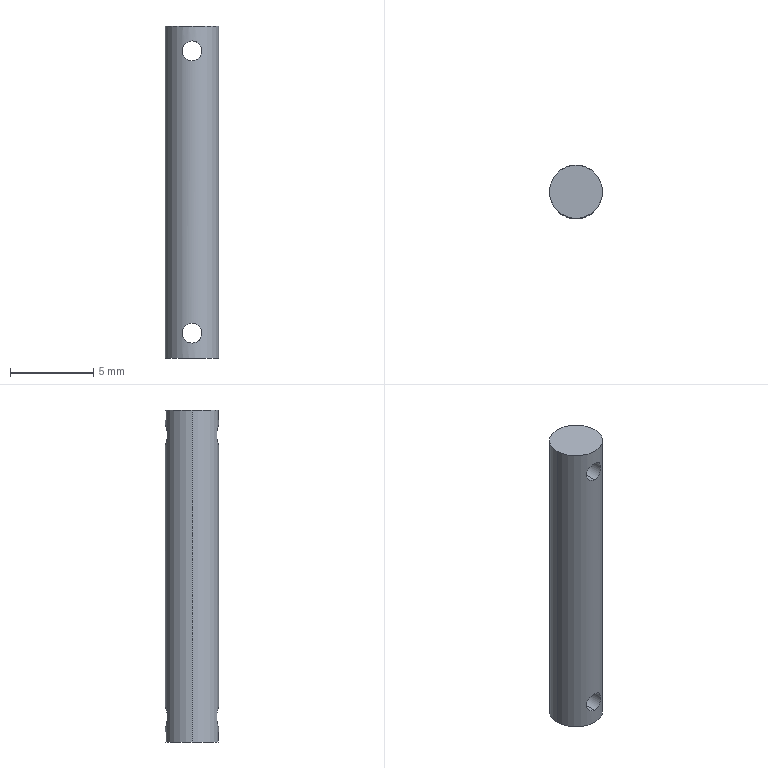Part | SolidWorks | features BaseBody 1 | 1 solid | 8 faces | box 3.2 x 3.2 x 20 mm | volume 153.742 mm3 | cylinder 6 | plane 2 | commonest cylinder face diameters 1.2 x4 3.2 x2
STEP:
#1=CARTESIAN_POINT('',(0.,-1.6,0.9));
#2=VERTEX_POINT('',#1);
#3=CARTESIAN_POINT('',(0.,1.6,0.9));
#4=VERTEX_POINT('',#3);
#5=CARTESIAN_POINT('',(0.,-1.6,0.9));
#6=DIRECTION('',(0.,1.,0.));
#7=VECTOR('',#6,1000.);
#8=LINE('',#5,#7);
#9=EDGE_CURVE('',#2,#4,#8,.T.);
#10=ORIENTED_EDGE('',*,*,#9,.F.);
#11=CARTESIAN_POINT('',(0.,-1.6,2.1));
#12=VERTEX_POINT('',#11);
#13=CARTESIAN_POINT('',(0.,-1.6,2.1));
#14=CARTESIAN_POINT('',(0.0792,-1.6,2.1));
#15=CARTESIAN_POINT('',(0.1577,-1.594,2.084));
#16=CARTESIAN_POINT('',(0.3049,-1.572,2.022));
#17=CARTESIAN_POINT('',(0.3691,-1.558,1.979));
#18=CARTESIAN_POINT('',(0.4799,-1.527,1.869));
#19=CARTESIAN_POINT('',(0.5219,-1.513,1.806));
#20=CARTESIAN_POINT('',(0.5845,-1.49,1.655));
#21=CARTESIAN_POINT('',(0.5999,-1.483,1.578));
#22=CARTESIAN_POINT('',(0.6001,-1.483,1.422));
#23=CARTESIAN_POINT('',(0.584,-1.49,1.344));
#24=CARTESIAN_POINT('',(0.5225,-1.513,1.196));
#25=CARTESIAN_POINT('',(0.48,-1.527,1.131));
#26=CARTESIAN_POINT('',(0.3682,-1.558,1.02));
#27=CARTESIAN_POINT('',(0.3045,-1.573,0.9769));
#28=CARTESIAN_POINT('',(0.1569,-1.594,0.9154));
#29=CARTESIAN_POINT('',(0.07976,-1.6,0.9));
#30=CARTESIAN_POINT('',(0.,-1.6,0.9));
#31=B_SPLINE_CURVE_WITH_KNOTS('',3,(#13,#14,#15,#16,#17,#18,#19,#20,#21,#22,#23,#24,#25,#26,#27,#28,#29,#30),.UNSPECIFIED.,.F.,.F.,(4,2,2,2,2,2,2,2,4),(0.,0.125,0.25,0.375,0.5,0.625,0.75,0.875,1.),.UNSPECIFIED.);
#32=EDGE_CURVE('',#12,#2,#31,.T.);
#33=ORIENTED_EDGE('',*,*,#32,.F.);
#34=CARTESIAN_POINT('',(0.,1.6,2.1));
#35=VERTEX_POINT('',#34);
#36=CARTESIAN_POINT('',(0.,-1.6,2.1));
#37=DIRECTION('',(0.,1.,0.));
#38=VECTOR('',#37,1000.);
#39=LINE('',#36,#38);
#40=EDGE_CURVE('',#12,#35,#39,.T.);
#41=ORIENTED_EDGE('',*,*,#40,.T.);
#42=CARTESIAN_POINT('',(0.,1.6,0.9));
#43=CARTESIAN_POINT('',(0.07978,1.6,0.9));
#44=CARTESIAN_POINT('',(0.1578,1.594,0.9157));
#45=CARTESIAN_POINT('',(0.304,1.573,0.9767));
#46=CARTESIAN_POINT('',(0.3682,1.558,1.02));
#47=CARTESIAN_POINT('',(0.4809,1.527,1.132));
#48=CARTESIAN_POINT('',(0.5232,1.512,1.195));
#49=CARTESIAN_POINT('',(0.5848,1.49,1.344));
#50=CARTESIAN_POINT('',(0.6,1.483,1.422));
#51=CARTESIAN_POINT('',(0.6,1.483,1.578));
#52=CARTESIAN_POINT('',(0.5839,1.49,1.657));
#53=CARTESIAN_POINT('',(0.5225,1.513,1.804));
#54=CARTESIAN_POINT('',(0.4795,1.528,1.869));
#55=CARTESIAN_POINT('',(0.3687,1.558,1.98));
#56=CARTESIAN_POINT('',(0.3053,1.572,2.022));
#57=CARTESIAN_POINT('',(0.1565,1.594,2.084));
#58=CARTESIAN_POINT('',(0.07933,1.6,2.1));
#59=CARTESIAN_POINT('',(0.,1.6,2.1));
#60=B_SPLINE_CURVE_WITH_KNOTS('',3,(#42,#43,#44,#45,#46,#47,#48,#49,#50,#51,#52,#53,#54,#55,#56,#57,#58,#59),.UNSPECIFIED.,.F.,.F.,(4,2,2,2,2,2,2,2,4),(0.,0.125,0.25,0.375,0.5,0.625,0.75,0.875,1.),.UNSPECIFIED.);
#61=EDGE_CURVE('',#4,#35,#60,.T.);
#62=ORIENTED_EDGE('',*,*,#61,.F.);
#63=EDGE_LOOP('',(#10,#33,#41,#62));
#64=FACE_OUTER_BOUND('',#63,.T.);
#65=CARTESIAN_POINT('',(0.,-1.6,1.5));
#66=DIRECTION('',(0.,1.,0.));
#67=DIRECTION('',(0.,0.,1.));
#68=AXIS2_PLACEMENT_3D('',#65,#66,#67);
#69=CYLINDRICAL_SURFACE('',#68,0.6);
#70=ADVANCED_FACE('',(#64),#69,.F.);
#71=CARTESIAN_POINT('',(0.,-1.6,17.9));
#72=VERTEX_POINT('',#71);
#73=CARTESIAN_POINT('',(0.,1.6,17.9));
#74=VERTEX_POINT('',#73);
#75=CARTESIAN_POINT('',(0.,-1.6,17.9));
#76=DIRECTION('',(0.,1.,0.));
#77=VECTOR('',#76,1000.);
#78=LINE('',#75,#77);
#79=EDGE_CURVE('',#72,#74,#78,.T.);
#80=ORIENTED_EDGE('',*,*,#79,.F.);
#81=CARTESIAN_POINT('',(0.,-1.6,19.1));
#82=VERTEX_POINT('',#81);
#83=CARTESIAN_POINT('',(0.,-1.6,19.1));
#84=CARTESIAN_POINT('',(0.0792,-1.6,19.1));
#85=CARTESIAN_POINT('',(0.1577,-1.594,19.084));
#86=CARTESIAN_POINT('',(0.3049,-1.572,19.022));
#87=CARTESIAN_POINT('',(0.3691,-1.558,18.979));
#88=CARTESIAN_POINT('',(0.4799,-1.527,18.869));
#89=CARTESIAN_POINT('',(0.5219,-1.513,18.806));
#90=CARTESIAN_POINT('',(0.5845,-1.49,18.655));
#91=CARTESIAN_POINT('',(0.5999,-1.483,18.578));
#92=CARTESIAN_POINT('',(0.6001,-1.483,18.422));
#93=CARTESIAN_POINT('',(0.584,-1.49,18.344));
#94=CARTESIAN_POINT('',(0.5225,-1.513,18.196));
#95=CARTESIAN_POINT('',(0.48,-1.527,18.131));
#96=CARTESIAN_POINT('',(0.3682,-1.558,18.02));
#97=CARTESIAN_POINT('',(0.3045,-1.573,17.977));
#98=CARTESIAN_POINT('',(0.1569,-1.594,17.915));
#99=CARTESIAN_POINT('',(0.07976,-1.6,17.9));
#100=CARTESIAN_POINT('',(0.,-1.6,17.9));
#101=B_SPLINE_CURVE_WITH_KNOTS('',3,(#83,#84,#85,#86,#87,#88,#89,#90,#91,#92,#93,#94,#95,#96,#97,#98,#99,#100),.UNSPECIFIED.,.F.,.F.,(4,2,2,2,2,2,2,2,4),(0.,0.125,0.25,0.375,0.5,0.625,0.75,0.875,1.),.UNSPECIFIED.);
#102=EDGE_CURVE('',#82,#72,#101,.T.);
#103=ORIENTED_EDGE('',*,*,#102,.F.);
#104=CARTESIAN_POINT('',(0.,1.6,19.1));
#105=VERTEX_POINT('',#104);
#106=CARTESIAN_POINT('',(0.,-1.6,19.1));
#107=DIRECTION('',(0.,1.,0.));
#108=VECTOR('',#107,1000.);
#109=LINE('',#106,#108);
#110=EDGE_CURVE('',#82,#105,#109,.T.);
#111=ORIENTED_EDGE('',*,*,#110,.T.);
#112=CARTESIAN_POINT('',(0.,1.6,17.9));
#113=CARTESIAN_POINT('',(0.07978,1.6,17.9));
#114=CARTESIAN_POINT('',(0.1578,1.594,17.916));
#115=CARTESIAN_POINT('',(0.304,1.573,17.977));
#116=CARTESIAN_POINT('',(0.3682,1.558,18.02));
#117=CARTESIAN_POINT('',(0.4809,1.527,18.132));
#118=CARTESIAN_POINT('',(0.5232,1.512,18.195));
#119=CARTESIAN_POINT('',(0.5848,1.49,18.344));
#120=CARTESIAN_POINT('',(0.6,1.483,18.422));
#121=CARTESIAN_POINT('',(0.6,1.483,18.578));
#122=CARTESIAN_POINT('',(0.5839,1.49,18.657));
#123=CARTESIAN_POINT('',(0.5225,1.513,18.804));
#124=CARTESIAN_POINT('',(0.4795,1.528,18.869));
#125=CARTESIAN_POINT('',(0.3687,1.558,18.98));
#126=CARTESIAN_POINT('',(0.3053,1.572,19.022));
#127=CARTESIAN_POINT('',(0.1565,1.594,19.084));
#128=CARTESIAN_POINT('',(0.07933,1.6,19.1));
#129=CARTESIAN_POINT('',(0.,1.6,19.1));
#130=B_SPLINE_CURVE_WITH_KNOTS('',3,(#112,#113,#114,#115,#116,#117,#118,#119,#120,#121,#122,#123,#124,#125,#126,#127,#128,#129),.UNSPECIFIED.,.F.,.F.,(4,2,2,2,2,2,2,2,4),(0.,0.125,0.25,0.375,0.5,0.625,0.75,0.875,1.),.UNSPECIFIED.);
#131=EDGE_CURVE('',#74,#105,#130,.T.);
#132=ORIENTED_EDGE('',*,*,#131,.F.);
#133=EDGE_LOOP('',(#80,#103,#111,#132));
#134=FACE_OUTER_BOUND('',#133,.T.);
#135=CARTESIAN_POINT('',(0.,-1.6,18.5));
#136=DIRECTION('',(0.,1.,0.));
#137=DIRECTION('',(0.,0.,1.));
#138=AXIS2_PLACEMENT_3D('',#135,#136,#137);
#139=CYLINDRICAL_SURFACE('',#138,0.6);
#140=ADVANCED_FACE('',(#134),#139,.F.);
#141=CARTESIAN_POINT('',(-1.6,0.,0.));
#142=VERTEX_POINT('',#141);
#143=CARTESIAN_POINT('',(1.6,0.,0.));
#144=VERTEX_POINT('',#143);
#145=CARTESIAN_POINT('',(0.,0.,0.));
#146=DIRECTION('',(0.,0.,1.));
#147=DIRECTION('',(1.,0.,0.));
#148=AXIS2_PLACEMENT_3D('',#145,#146,#147);
#149=CIRCLE('',#148,1.6);
#150=EDGE_CURVE('',#142,#144,#149,.T.);
#151=ORIENTED_EDGE('',*,*,#150,.F.);
#152=CARTESIAN_POINT('',(0.,0.,0.));
#153=DIRECTION('',(0.,0.,1.));
#154=DIRECTION('',(1.,0.,0.));
#155=AXIS2_PLACEMENT_3D('',#152,#153,#154);
#156=CIRCLE('',#155,1.6);
#157=EDGE_CURVE('',#144,#142,#156,.T.);
#158=ORIENTED_EDGE('',*,*,#157,.F.);
#159=EDGE_LOOP('',(#151,#158));
#160=FACE_OUTER_BOUND('',#159,.T.);
#161=CARTESIAN_POINT('',(0.,0.,0.));
#162=DIRECTION('',(0.,0.,1.));
#163=DIRECTION('',(1.,0.,0.));
#164=AXIS2_PLACEMENT_3D('',#161,#162,#163);
#165=PLANE('',#164);
#166=ADVANCED_FACE('',(#160),#165,.F.);
#167=CARTESIAN_POINT('',(-1.6,0.,20.));
#168=VERTEX_POINT('',#167);
#169=CARTESIAN_POINT('',(1.6,0.,20.));
#170=VERTEX_POINT('',#169);
#171=CARTESIAN_POINT('',(0.,0.,20.));
#172=DIRECTION('',(0.,0.,1.));
#173=DIRECTION('',(1.,0.,0.));
#174=AXIS2_PLACEMENT_3D('',#171,#172,#173);
#175=CIRCLE('',#174,1.6);
#176=EDGE_CURVE('',#168,#170,#175,.T.);
#177=ORIENTED_EDGE('',*,*,#176,.T.);
#178=CARTESIAN_POINT('',(0.,0.,20.));
#179=DIRECTION('',(0.,0.,1.));
#180=DIRECTION('',(1.,0.,0.));
#181=AXIS2_PLACEMENT_3D('',#178,#179,#180);
#182=CIRCLE('',#181,1.6);
#183=EDGE_CURVE('',#170,#168,#182,.T.);
#184=ORIENTED_EDGE('',*,*,#183,.T.);
#185=EDGE_LOOP('',(#177,#184));
#186=FACE_OUTER_BOUND('',#185,.T.);
#187=CARTESIAN_POINT('',(0.,0.,20.));
#188=DIRECTION('',(0.,0.,1.));
#189=DIRECTION('',(1.,0.,0.));
#190=AXIS2_PLACEMENT_3D('',#187,#188,#189);
#191=PLANE('',#190);
#192=ADVANCED_FACE('',(#186),#191,.T.);
#193=ORIENTED_EDGE('',*,*,#102,.T.);
#194=CARTESIAN_POINT('',(0.,-1.6,17.9));
#195=CARTESIAN_POINT('',(-0.07978,-1.6,17.9));
#196=CARTESIAN_POINT('',(-0.1578,-1.594,17.916));
#197=CARTESIAN_POINT('',(-0.304,-1.573,17.977));
#198=CARTESIAN_POINT('',(-0.3682,-1.558,18.02));
#199=CARTESIAN_POINT('',(-0.4809,-1.527,18.132));
#200=CARTESIAN_POINT('',(-0.5232,-1.512,18.195));
#201=CARTESIAN_POINT('',(-0.5848,-1.49,18.344));
#202=CARTESIAN_POINT('',(-0.6,-1.483,18.422));
#203=CARTESIAN_POINT('',(-0.6,-1.483,18.578));
#204=CARTESIAN_POINT('',(-0.5839,-1.49,18.657));
#205=CARTESIAN_POINT('',(-0.5225,-1.513,18.804));
#206=CARTESIAN_POINT('',(-0.4795,-1.528,18.869));
#207=CARTESIAN_POINT('',(-0.3687,-1.558,18.98));
#208=CARTESIAN_POINT('',(-0.3053,-1.572,19.022));
#209=CARTESIAN_POINT('',(-0.1565,-1.594,19.084));
#210=CARTESIAN_POINT('',(-0.07933,-1.6,19.1));
#211=CARTESIAN_POINT('',(0.,-1.6,19.1));
#212=B_SPLINE_CURVE_WITH_KNOTS('',3,(#194,#195,#196,#197,#198,#199,#200,#201,#202,#203,#204,#205,#206,#207,#208,#209,#210,#211),.UNSPECIFIED.,.F.,.F.,(4,2,2,2,2,2,2,2,4),(0.,0.125,0.25,0.375,0.5,0.625,0.75,0.875,1.),.UNSPECIFIED.);
#213=EDGE_CURVE('',#72,#82,#212,.T.);
#214=ORIENTED_EDGE('',*,*,#213,.T.);
#215=EDGE_LOOP('',(#193,#214));
#216=FACE_BOUND('',#215,.T.);
#217=ORIENTED_EDGE('',*,*,#32,.T.);
#218=CARTESIAN_POINT('',(0.,-1.6,0.9));
#219=CARTESIAN_POINT('',(-0.07978,-1.6,0.9));
#220=CARTESIAN_POINT('',(-0.1578,-1.594,0.9157));
#221=CARTESIAN_POINT('',(-0.304,-1.573,0.9767));
#222=CARTESIAN_POINT('',(-0.3682,-1.558,1.02));
#223=CARTESIAN_POINT('',(-0.4809,-1.527,1.132));
#224=CARTESIAN_POINT('',(-0.5232,-1.512,1.195));
#225=CARTESIAN_POINT('',(-0.5848,-1.49,1.344));
#226=CARTESIAN_POINT('',(-0.6,-1.483,1.422));
#227=CARTESIAN_POINT('',(-0.6,-1.483,1.578));
#228=CARTESIAN_POINT('',(-0.5839,-1.49,1.657));
#229=CARTESIAN_POINT('',(-0.5225,-1.513,1.804));
#230=CARTESIAN_POINT('',(-0.4795,-1.528,1.869));
#231=CARTESIAN_POINT('',(-0.3687,-1.558,1.98));
#232=CARTESIAN_POINT('',(-0.3053,-1.572,2.022));
#233=CARTESIAN_POINT('',(-0.1565,-1.594,2.084));
#234=CARTESIAN_POINT('',(-0.07933,-1.6,2.1));
#235=CARTESIAN_POINT('',(0.,-1.6,2.1));
#236=B_SPLINE_CURVE_WITH_KNOTS('',3,(#218,#219,#220,#221,#222,#223,#224,#225,#226,#227,#228,#229,#230,#231,#232,#233,#234,#235),.UNSPECIFIED.,.F.,.F.,(4,2,2,2,2,2,2,2,4),(0.,0.125,0.25,0.375,0.5,0.625,0.75,0.875,1.),.UNSPECIFIED.);
#237=EDGE_CURVE('',#2,#12,#236,.T.);
#238=ORIENTED_EDGE('',*,*,#237,.T.);
#239=EDGE_LOOP('',(#217,#238));
#240=FACE_BOUND('',#239,.T.);
#241=CARTESIAN_POINT('',(1.6,0.,20.));
#242=DIRECTION('',(0.,0.,-1.));
#243=VECTOR('',#242,1000.);
#244=LINE('',#241,#243);
#245=EDGE_CURVE('',#170,#144,#244,.T.);
#246=ORIENTED_EDGE('',*,*,#245,.F.);
#247=ORIENTED_EDGE('',*,*,#176,.F.);
#248=CARTESIAN_POINT('',(-1.6,0.,20.));
#249=DIRECTION('',(0.,0.,-1.));
#250=VECTOR('',#249,1000.);
#251=LINE('',#248,#250);
#252=EDGE_CURVE('',#168,#142,#251,.T.);
#253=ORIENTED_EDGE('',*,*,#252,.T.);
#254=ORIENTED_EDGE('',*,*,#150,.T.);
#255=EDGE_LOOP('',(#246,#247,#253,#254));
#256=FACE_OUTER_BOUND('',#255,.T.);
#257=CARTESIAN_POINT('',(0.,0.,20.));
#258=DIRECTION('',(0.,0.,-1.));
#259=DIRECTION('',(-1.,0.,0.));
#260=AXIS2_PLACEMENT_3D('',#257,#258,#259);
#261=CYLINDRICAL_SURFACE('',#260,1.6);
#262=ADVANCED_FACE('',(#216,#240,#256),#261,.T.);
#263=CARTESIAN_POINT('',(0.,1.6,2.1));
#264=CARTESIAN_POINT('',(-0.0792,1.6,2.1));
#265=CARTESIAN_POINT('',(-0.1577,1.594,2.084));
#266=CARTESIAN_POINT('',(-0.3049,1.572,2.022));
#267=CARTESIAN_POINT('',(-0.3691,1.558,1.979));
#268=CARTESIAN_POINT('',(-0.4799,1.527,1.869));
#269=CARTESIAN_POINT('',(-0.5219,1.513,1.806));
#270=CARTESIAN_POINT('',(-0.5845,1.49,1.655));
#271=CARTESIAN_POINT('',(-0.5999,1.483,1.578));
#272=CARTESIAN_POINT('',(-0.6001,1.483,1.422));
#273=CARTESIAN_POINT('',(-0.584,1.49,1.344));
#274=CARTESIAN_POINT('',(-0.5225,1.513,1.196));
#275=CARTESIAN_POINT('',(-0.48,1.527,1.131));
#276=CARTESIAN_POINT('',(-0.3682,1.558,1.02));
#277=CARTESIAN_POINT('',(-0.3045,1.573,0.9769));
#278=CARTESIAN_POINT('',(-0.1569,1.594,0.9154));
#279=CARTESIAN_POINT('',(-0.07976,1.6,0.9));
#280=CARTESIAN_POINT('',(0.,1.6,0.9));
#281=B_SPLINE_CURVE_WITH_KNOTS('',3,(#263,#264,#265,#266,#267,#268,#269,#270,#271,#272,#273,#274,#275,#276,#277,#278,#279,#280),.UNSPECIFIED.,.F.,.F.,(4,2,2,2,2,2,2,2,4),(0.,0.125,0.25,0.375,0.5,0.625,0.75,0.875,1.),.UNSPECIFIED.);
#282=EDGE_CURVE('',#35,#4,#281,.T.);
#283=ORIENTED_EDGE('',*,*,#282,.T.);
#284=ORIENTED_EDGE('',*,*,#61,.T.);
#285=EDGE_LOOP('',(#283,#284));
#286=FACE_BOUND('',#285,.T.);
#287=CARTESIAN_POINT('',(0.,1.6,19.1));
#288=CARTESIAN_POINT('',(-0.0792,1.6,19.1));
#289=CARTESIAN_POINT('',(-0.1577,1.594,19.084));
#290=CARTESIAN_POINT('',(-0.3049,1.572,19.022));
#291=CARTESIAN_POINT('',(-0.3691,1.558,18.979));
#292=CARTESIAN_POINT('',(-0.4799,1.527,18.869));
#293=CARTESIAN_POINT('',(-0.5219,1.513,18.806));
#294=CARTESIAN_POINT('',(-0.5845,1.49,18.655));
#295=CARTESIAN_POINT('',(-0.5999,1.483,18.578));
#296=CARTESIAN_POINT('',(-0.6001,1.483,18.422));
#297=CARTESIAN_POINT('',(-0.584,1.49,18.344));
#298=CARTESIAN_POINT('',(-0.5225,1.513,18.196));
#299=CARTESIAN_POINT('',(-0.48,1.527,18.131));
#300=CARTESIAN_POINT('',(-0.3682,1.558,18.02));
#301=CARTESIAN_POINT('',(-0.3045,1.573,17.977));
#302=CARTESIAN_POINT('',(-0.1569,1.594,17.915));
#303=CARTESIAN_POINT('',(-0.07976,1.6,17.9));
#304=CARTESIAN_POINT('',(0.,1.6,17.9));
#305=B_SPLINE_CURVE_WITH_KNOTS('',3,(#287,#288,#289,#290,#291,#292,#293,#294,#295,#296,#297,#298,#299,#300,#301,#302,#303,#304),.UNSPECIFIED.,.F.,.F.,(4,2,2,2,2,2,2,2,4),(0.,0.125,0.25,0.375,0.5,0.625,0.75,0.875,1.),.UNSPECIFIED.);
#306=EDGE_CURVE('',#105,#74,#305,.T.);
#307=ORIENTED_EDGE('',*,*,#306,.T.);
#308=ORIENTED_EDGE('',*,*,#131,.T.);
#309=EDGE_LOOP('',(#307,#308));
#310=FACE_BOUND('',#309,.T.);
#311=ORIENTED_EDGE('',*,*,#183,.F.);
#312=ORIENTED_EDGE('',*,*,#245,.T.);
#313=ORIENTED_EDGE('',*,*,#157,.T.);
#314=ORIENTED_EDGE('',*,*,#252,.F.);
#315=EDGE_LOOP('',(#311,#312,#313,#314));
#316=FACE_OUTER_BOUND('',#315,.T.);
#317=CARTESIAN_POINT('',(0.,0.,20.));
#318=DIRECTION('',(0.,0.,-1.));
#319=DIRECTION('',(-1.,0.,0.));
#320=AXIS2_PLACEMENT_3D('',#317,#318,#319);
#321=CYLINDRICAL_SURFACE('',#320,1.6);
#322=ADVANCED_FACE('',(#286,#310,#316),#321,.T.);
#323=ORIENTED_EDGE('',*,*,#213,.F.);
#324=ORIENTED_EDGE('',*,*,#79,.T.);
#325=ORIENTED_EDGE('',*,*,#306,.F.);
#326=ORIENTED_EDGE('',*,*,#110,.F.);
#327=EDGE_LOOP('',(#323,#324,#325,#326));
#328=FACE_OUTER_BOUND('',#327,.T.);
#329=CARTESIAN_POINT('',(0.,-1.6,18.5));
#330=DIRECTION('',(0.,1.,0.));
#331=DIRECTION('',(0.,0.,1.));
#332=AXIS2_PLACEMENT_3D('',#329,#330,#331);
#333=CYLINDRICAL_SURFACE('',#332,0.6);
#334=ADVANCED_FACE('',(#328),#333,.F.);
#335=ORIENTED_EDGE('',*,*,#237,.F.);
#336=ORIENTED_EDGE('',*,*,#9,.T.);
#337=ORIENTED_EDGE('',*,*,#282,.F.);
#338=ORIENTED_EDGE('',*,*,#40,.F.);
#339=EDGE_LOOP('',(#335,#336,#337,#338));
#340=FACE_OUTER_BOUND('',#339,.T.);
#341=CARTESIAN_POINT('',(0.,-1.6,1.5));
#342=DIRECTION('',(0.,1.,0.));
#343=DIRECTION('',(0.,0.,1.));
#344=AXIS2_PLACEMENT_3D('',#341,#342,#343);
#345=CYLINDRICAL_SURFACE('',#344,0.6);
#346=ADVANCED_FACE('',(#340),#345,.F.);
#347=CLOSED_SHELL('',(#70,#140,#166,#192,#262,#322,#334,#346));
#348=MANIFOLD_SOLID_BREP('',#347);
#349=CARTESIAN_POINT('',(0.,0.,0.));
#350=DIRECTION('',(0.,0.,1.));
#351=DIRECTION('',(1.,0.,0.));
#352=AXIS2_PLACEMENT_3D('',#349,#350,#351);
#353=(LENGTH_UNIT()NAMED_UNIT(*)SI_UNIT(.MILLI.,.METRE.));
#354=UNCERTAINTY_MEASURE_WITH_UNIT(LENGTH_MEASURE(0.00001),#353,'','');
#355=(NAMED_UNIT(*)PLANE_ANGLE_UNIT()SI_UNIT($,.RADIAN.));
#356=(NAMED_UNIT(*)SI_UNIT($,.STERADIAN.)SOLID_ANGLE_UNIT());
#357=(GEOMETRIC_REPRESENTATION_CONTEXT(3)GLOBAL_UNCERTAINTY_ASSIGNED_CONTEXT((#354))GLOBAL_UNIT_ASSIGNED_CONTEXT((#353,#355,#356))REPRESENTATION_CONTEXT('',''));
#358=ADVANCED_BREP_SHAPE_REPRESENTATION('',(#348,#352),#357);